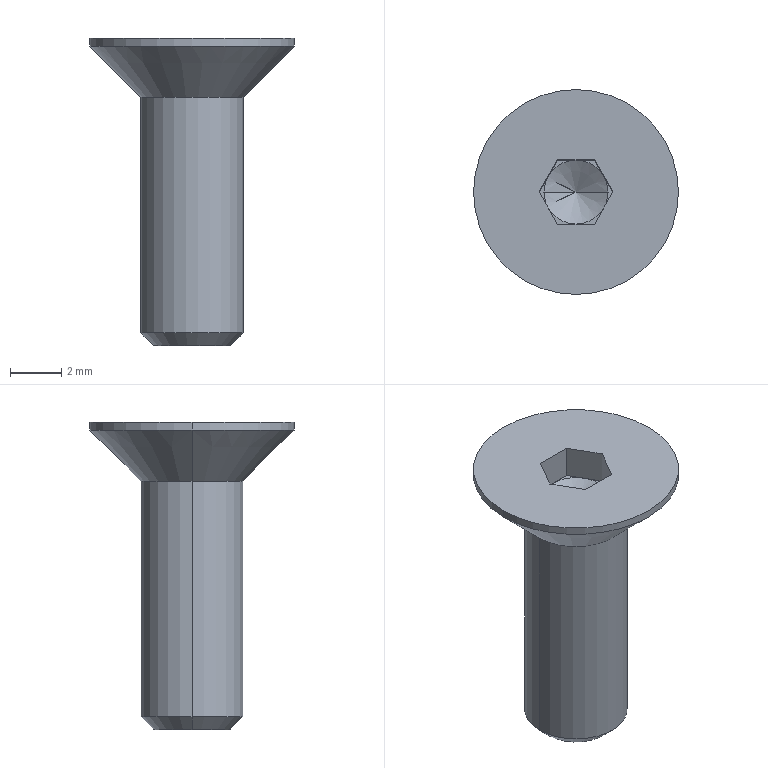Part | NX | features BREP 1 | 1 solid | 24 faces | box 8 x 8 x 12 mm | volume 185.959 mm3 | plane 14 | cone 6 | cylinder 4 | commonest cylinder face diameters 4 x2 8 x2
STEP:
#1=CARTESIAN_POINT('',(0.,0.,-2.022));
#2=VERTEX_POINT('',#1);
#3=CARTESIAN_POINT('',(-1.25,0.,-1.3));
#4=VERTEX_POINT('',#3);
#5=CARTESIAN_POINT('',(-1.25,0.,-1.3));
#6=DIRECTION('',(-0.866,0.,0.5));
#7=VECTOR('',#6,1000.);
#8=LINE('',#5,#7);
#9=EDGE_CURVE('',#2,#4,#8,.T.);
#10=ORIENTED_EDGE('',*,*,#9,.F.);
#11=CARTESIAN_POINT('',(1.25,0.,-1.3));
#12=VERTEX_POINT('',#11);
#13=CARTESIAN_POINT('',(1.25,0.,-1.3));
#14=DIRECTION('',(0.866,0.,0.5));
#15=VECTOR('',#14,1000.);
#16=LINE('',#13,#15);
#17=EDGE_CURVE('',#2,#12,#16,.T.);
#18=ORIENTED_EDGE('',*,*,#17,.T.);
#19=CARTESIAN_POINT('',(1.083,0.625,-1.3));
#20=VERTEX_POINT('',#19);
#21=CARTESIAN_POINT('',(0.,0.,-1.3));
#22=DIRECTION('',(0.,0.,-1.));
#23=DIRECTION('',(-1.,0.,0.));
#24=AXIS2_PLACEMENT_3D('',#21,#22,#23);
#25=CIRCLE('',#24,1.25);
#26=EDGE_CURVE('',#20,#12,#25,.T.);
#27=ORIENTED_EDGE('',*,*,#26,.F.);
#28=CARTESIAN_POINT('',(0.,1.25,-1.3));
#29=VERTEX_POINT('',#28);
#30=CARTESIAN_POINT('',(0.,0.,-1.3));
#31=DIRECTION('',(0.,0.,-1.));
#32=DIRECTION('',(-1.,0.,0.));
#33=AXIS2_PLACEMENT_3D('',#30,#31,#32);
#34=CIRCLE('',#33,1.25);
#35=EDGE_CURVE('',#29,#20,#34,.T.);
#36=ORIENTED_EDGE('',*,*,#35,.F.);
#37=CARTESIAN_POINT('',(-1.083,0.625,-1.3));
#38=VERTEX_POINT('',#37);
#39=CARTESIAN_POINT('',(0.,0.,-1.3));
#40=DIRECTION('',(0.,0.,-1.));
#41=DIRECTION('',(-1.,0.,0.));
#42=AXIS2_PLACEMENT_3D('',#39,#40,#41);
#43=CIRCLE('',#42,1.25);
#44=EDGE_CURVE('',#38,#29,#43,.T.);
#45=ORIENTED_EDGE('',*,*,#44,.F.);
#46=CARTESIAN_POINT('',(0.,0.,-1.3));
#47=DIRECTION('',(0.,0.,-1.));
#48=DIRECTION('',(-1.,0.,0.));
#49=AXIS2_PLACEMENT_3D('',#46,#47,#48);
#50=CIRCLE('',#49,1.25);
#51=EDGE_CURVE('',#4,#38,#50,.T.);
#52=ORIENTED_EDGE('',*,*,#51,.F.);
#53=EDGE_LOOP('',(#10,#18,#27,#36,#45,#52));
#54=FACE_BOUND('',#53,.T.);
#55=CARTESIAN_POINT('',(0.,0.,-1.3));
#56=DIRECTION('',(0.,0.,1.));
#57=DIRECTION('',(-1.,0.,0.));
#58=AXIS2_PLACEMENT_3D('',#55,#56,#57);
#59=CONICAL_SURFACE('',#58,1.25,1.047);
#60=ADVANCED_FACE('',(#54),#59,.F.);
#61=CARTESIAN_POINT('',(-1.5,0.,-12.));
#62=VERTEX_POINT('',#61);
#63=CARTESIAN_POINT('',(1.5,0.,-12.));
#64=VERTEX_POINT('',#63);
#65=CARTESIAN_POINT('',(0.,0.,-12.));
#66=DIRECTION('',(0.,0.,1.));
#67=DIRECTION('',(1.,0.,0.));
#68=AXIS2_PLACEMENT_3D('',#65,#66,#67);
#69=CIRCLE('',#68,1.5);
#70=EDGE_CURVE('',#62,#64,#69,.T.);
#71=ORIENTED_EDGE('',*,*,#70,.T.);
#72=CARTESIAN_POINT('',(2.,0.,-11.5));
#73=VERTEX_POINT('',#72);
#74=CARTESIAN_POINT('',(1.5,0.,-12.));
#75=DIRECTION('',(0.7071,0.,0.7071));
#76=VECTOR('',#75,1000.);
#77=LINE('',#74,#76);
#78=EDGE_CURVE('',#64,#73,#77,.T.);
#79=ORIENTED_EDGE('',*,*,#78,.T.);
#80=CARTESIAN_POINT('',(-2.,0.,-11.5));
#81=VERTEX_POINT('',#80);
#82=CARTESIAN_POINT('',(0.,0.,-11.5));
#83=DIRECTION('',(0.,0.,-1.));
#84=DIRECTION('',(1.,0.,0.));
#85=AXIS2_PLACEMENT_3D('',#82,#83,#84);
#86=CIRCLE('',#85,2.);
#87=EDGE_CURVE('',#73,#81,#86,.T.);
#88=ORIENTED_EDGE('',*,*,#87,.T.);
#89=CARTESIAN_POINT('',(-1.5,0.,-12.));
#90=DIRECTION('',(-0.7071,0.,0.7071));
#91=VECTOR('',#90,1000.);
#92=LINE('',#89,#91);
#93=EDGE_CURVE('',#62,#81,#92,.T.);
#94=ORIENTED_EDGE('',*,*,#93,.F.);
#95=EDGE_LOOP('',(#71,#79,#88,#94));
#96=FACE_BOUND('',#95,.T.);
#97=CARTESIAN_POINT('',(0.,0.,-12.));
#98=DIRECTION('',(0.,0.,1.));
#99=DIRECTION('',(-1.,0.,0.));
#100=AXIS2_PLACEMENT_3D('',#97,#98,#99);
#101=CONICAL_SURFACE('',#100,1.5,0.7854);
#102=ADVANCED_FACE('',(#96),#101,.T.);
#103=ORIENTED_EDGE('',*,*,#87,.F.);
#104=CARTESIAN_POINT('',(2.,0.,-2.3));
#105=VERTEX_POINT('',#104);
#106=CARTESIAN_POINT('',(2.,0.,-12.));
#107=DIRECTION('',(0.,0.,1.));
#108=VECTOR('',#107,1000.);
#109=LINE('',#106,#108);
#110=EDGE_CURVE('',#73,#105,#109,.T.);
#111=ORIENTED_EDGE('',*,*,#110,.T.);
#112=CARTESIAN_POINT('',(-2.,0.,-2.3));
#113=VERTEX_POINT('',#112);
#114=CARTESIAN_POINT('',(0.,0.,-2.3));
#115=DIRECTION('',(0.,0.,1.));
#116=DIRECTION('',(1.,0.,0.));
#117=AXIS2_PLACEMENT_3D('',#114,#115,#116);
#118=CIRCLE('',#117,2.);
#119=EDGE_CURVE('',#113,#105,#118,.T.);
#120=ORIENTED_EDGE('',*,*,#119,.F.);
#121=CARTESIAN_POINT('',(-2.,0.,-12.));
#122=DIRECTION('',(0.,0.,1.));
#123=VECTOR('',#122,1000.);
#124=LINE('',#121,#123);
#125=EDGE_CURVE('',#81,#113,#124,.T.);
#126=ORIENTED_EDGE('',*,*,#125,.F.);
#127=EDGE_LOOP('',(#103,#111,#120,#126));
#128=FACE_BOUND('',#127,.T.);
#129=CARTESIAN_POINT('',(0.,0.,-12.));
#130=DIRECTION('',(0.,0.,1.));
#131=DIRECTION('',(-1.,0.,0.));
#132=AXIS2_PLACEMENT_3D('',#129,#130,#131);
#133=CYLINDRICAL_SURFACE('',#132,2.);
#134=ADVANCED_FACE('',(#128),#133,.T.);
#135=ORIENTED_EDGE('',*,*,#119,.T.);
#136=CARTESIAN_POINT('',(4.,0.,-0.3));
#137=VERTEX_POINT('',#136);
#138=CARTESIAN_POINT('',(2.,0.,-2.3));
#139=DIRECTION('',(0.7071,0.,0.7071));
#140=VECTOR('',#139,1000.);
#141=LINE('',#138,#140);
#142=EDGE_CURVE('',#105,#137,#141,.T.);
#143=ORIENTED_EDGE('',*,*,#142,.T.);
#144=CARTESIAN_POINT('',(-4.,0.,-0.3));
#145=VERTEX_POINT('',#144);
#146=CARTESIAN_POINT('',(0.,0.,-0.3));
#147=DIRECTION('',(0.,0.,-1.));
#148=DIRECTION('',(1.,0.,0.));
#149=AXIS2_PLACEMENT_3D('',#146,#147,#148);
#150=CIRCLE('',#149,4.);
#151=EDGE_CURVE('',#137,#145,#150,.T.);
#152=ORIENTED_EDGE('',*,*,#151,.T.);
#153=CARTESIAN_POINT('',(-2.,0.,-2.3));
#154=DIRECTION('',(-0.7071,0.,0.7071));
#155=VECTOR('',#154,1000.);
#156=LINE('',#153,#155);
#157=EDGE_CURVE('',#113,#145,#156,.T.);
#158=ORIENTED_EDGE('',*,*,#157,.F.);
#159=EDGE_LOOP('',(#135,#143,#152,#158));
#160=FACE_BOUND('',#159,.T.);
#161=CARTESIAN_POINT('',(0.,0.,-2.3));
#162=DIRECTION('',(0.,0.,1.));
#163=DIRECTION('',(-1.,0.,0.));
#164=AXIS2_PLACEMENT_3D('',#161,#162,#163);
#165=CONICAL_SURFACE('',#164,2.,0.7854);
#166=ADVANCED_FACE('',(#160),#165,.T.);
#167=ORIENTED_EDGE('',*,*,#151,.F.);
#168=CARTESIAN_POINT('',(4.,0.,0.));
#169=VERTEX_POINT('',#168);
#170=CARTESIAN_POINT('',(4.,0.,-2.3));
#171=DIRECTION('',(0.,0.,1.));
#172=VECTOR('',#171,1000.);
#173=LINE('',#170,#172);
#174=EDGE_CURVE('',#137,#169,#173,.T.);
#175=ORIENTED_EDGE('',*,*,#174,.T.);
#176=CARTESIAN_POINT('',(-4.,0.,0.));
#177=VERTEX_POINT('',#176);
#178=CARTESIAN_POINT('',(0.,0.,0.));
#179=DIRECTION('',(0.,0.,1.));
#180=DIRECTION('',(1.,0.,0.));
#181=AXIS2_PLACEMENT_3D('',#178,#179,#180);
#182=CIRCLE('',#181,4.);
#183=EDGE_CURVE('',#177,#169,#182,.T.);
#184=ORIENTED_EDGE('',*,*,#183,.F.);
#185=CARTESIAN_POINT('',(-4.,0.,-2.3));
#186=DIRECTION('',(0.,0.,1.));
#187=VECTOR('',#186,1000.);
#188=LINE('',#185,#187);
#189=EDGE_CURVE('',#145,#177,#188,.T.);
#190=ORIENTED_EDGE('',*,*,#189,.F.);
#191=EDGE_LOOP('',(#167,#175,#184,#190));
#192=FACE_BOUND('',#191,.T.);
#193=CARTESIAN_POINT('',(0.,0.,-2.3));
#194=DIRECTION('',(0.,0.,1.));
#195=DIRECTION('',(-1.,0.,0.));
#196=AXIS2_PLACEMENT_3D('',#193,#194,#195);
#197=CYLINDRICAL_SURFACE('',#196,4.);
#198=ADVANCED_FACE('',(#192),#197,.T.);
#199=ORIENTED_EDGE('',*,*,#44,.T.);
#200=CARTESIAN_POINT('',(-0.7217,1.25,-1.3));
#201=VERTEX_POINT('',#200);
#202=CARTESIAN_POINT('',(-0.7217,1.25,-1.3));
#203=DIRECTION('',(1.,0.,0.));
#204=VECTOR('',#203,1000.);
#205=LINE('',#202,#204);
#206=EDGE_CURVE('',#201,#29,#205,.T.);
#207=ORIENTED_EDGE('',*,*,#206,.F.);
#208=CARTESIAN_POINT('',(-1.443,0.,-1.3));
#209=DIRECTION('',(0.5,0.866,0.));
#210=VECTOR('',#209,1000.);
#211=LINE('',#208,#210);
#212=EDGE_CURVE('',#38,#201,#211,.T.);
#213=ORIENTED_EDGE('',*,*,#212,.F.);
#214=EDGE_LOOP('',(#199,#207,#213));
#215=FACE_BOUND('',#214,.T.);
#216=CARTESIAN_POINT('',(0.,0.,-1.3));
#217=DIRECTION('',(0.,0.,1.));
#218=DIRECTION('',(1.,0.,0.));
#219=AXIS2_PLACEMENT_3D('',#216,#217,#218);
#220=PLANE('',#219);
#221=ADVANCED_FACE('',(#215),#220,.T.);
#222=ORIENTED_EDGE('',*,*,#35,.T.);
#223=CARTESIAN_POINT('',(0.7217,1.25,-1.3));
#224=VERTEX_POINT('',#223);
#225=CARTESIAN_POINT('',(0.7217,1.25,-1.3));
#226=DIRECTION('',(0.5,-0.866,0.));
#227=VECTOR('',#226,1000.);
#228=LINE('',#225,#227);
#229=EDGE_CURVE('',#224,#20,#228,.T.);
#230=ORIENTED_EDGE('',*,*,#229,.F.);
#231=CARTESIAN_POINT('',(-0.7217,1.25,-1.3));
#232=DIRECTION('',(1.,0.,0.));
#233=VECTOR('',#232,1000.);
#234=LINE('',#231,#233);
#235=EDGE_CURVE('',#29,#224,#234,.T.);
#236=ORIENTED_EDGE('',*,*,#235,.F.);
#237=EDGE_LOOP('',(#222,#230,#236));
#238=FACE_BOUND('',#237,.T.);
#239=CARTESIAN_POINT('',(0.,0.,-1.3));
#240=DIRECTION('',(0.,0.,1.));
#241=DIRECTION('',(1.,0.,0.));
#242=AXIS2_PLACEMENT_3D('',#239,#240,#241);
#243=PLANE('',#242);
#244=ADVANCED_FACE('',(#238),#243,.T.);
#245=ORIENTED_EDGE('',*,*,#26,.T.);
#246=CARTESIAN_POINT('',(1.083,-0.625,-1.3));
#247=VERTEX_POINT('',#246);
#248=CARTESIAN_POINT('',(0.,0.,-1.3));
#249=DIRECTION('',(0.,0.,-1.));
#250=DIRECTION('',(-1.,0.,0.));
#251=AXIS2_PLACEMENT_3D('',#248,#249,#250);
#252=CIRCLE('',#251,1.25);
#253=EDGE_CURVE('',#12,#247,#252,.T.);
#254=ORIENTED_EDGE('',*,*,#253,.T.);
#255=CARTESIAN_POINT('',(1.443,0.,-1.3));
#256=VERTEX_POINT('',#255);
#257=CARTESIAN_POINT('',(1.443,0.,-1.3));
#258=DIRECTION('',(-0.5,-0.866,0.));
#259=VECTOR('',#258,1000.);
#260=LINE('',#257,#259);
#261=EDGE_CURVE('',#256,#247,#260,.T.);
#262=ORIENTED_EDGE('',*,*,#261,.F.);
#263=CARTESIAN_POINT('',(0.7217,1.25,-1.3));
#264=DIRECTION('',(0.5,-0.866,0.));
#265=VECTOR('',#264,1000.);
#266=LINE('',#263,#265);
#267=EDGE_CURVE('',#20,#256,#266,.T.);
#268=ORIENTED_EDGE('',*,*,#267,.F.);
#269=EDGE_LOOP('',(#245,#254,#262,#268));
#270=FACE_BOUND('',#269,.T.);
#271=CARTESIAN_POINT('',(0.,0.,-1.3));
#272=DIRECTION('',(0.,0.,1.));
#273=DIRECTION('',(1.,0.,0.));
#274=AXIS2_PLACEMENT_3D('',#271,#272,#273);
#275=PLANE('',#274);
#276=ADVANCED_FACE('',(#270),#275,.T.);
#277=CARTESIAN_POINT('',(0.,-1.25,-1.3));
#278=VERTEX_POINT('',#277);
#279=CARTESIAN_POINT('',(0.,0.,-1.3));
#280=DIRECTION('',(0.,0.,-1.));
#281=DIRECTION('',(-1.,0.,0.));
#282=AXIS2_PLACEMENT_3D('',#279,#280,#281);
#283=CIRCLE('',#282,1.25);
#284=EDGE_CURVE('',#247,#278,#283,.T.);
#285=ORIENTED_EDGE('',*,*,#284,.T.);
#286=CARTESIAN_POINT('',(0.7217,-1.25,-1.3));
#287=VERTEX_POINT('',#286);
#288=CARTESIAN_POINT('',(0.7217,-1.25,-1.3));
#289=DIRECTION('',(-1.,0.,0.));
#290=VECTOR('',#289,1000.);
#291=LINE('',#288,#290);
#292=EDGE_CURVE('',#287,#278,#291,.T.);
#293=ORIENTED_EDGE('',*,*,#292,.F.);
#294=CARTESIAN_POINT('',(1.443,0.,-1.3));
#295=DIRECTION('',(-0.5,-0.866,0.));
#296=VECTOR('',#295,1000.);
#297=LINE('',#294,#296);
#298=EDGE_CURVE('',#247,#287,#297,.T.);
#299=ORIENTED_EDGE('',*,*,#298,.F.);
#300=EDGE_LOOP('',(#285,#293,#299));
#301=FACE_BOUND('',#300,.T.);
#302=CARTESIAN_POINT('',(0.,0.,-1.3));
#303=DIRECTION('',(0.,0.,1.));
#304=DIRECTION('',(1.,0.,0.));
#305=AXIS2_PLACEMENT_3D('',#302,#303,#304);
#306=PLANE('',#305);
#307=ADVANCED_FACE('',(#301),#306,.T.);
#308=CARTESIAN_POINT('',(-1.083,-0.625,-1.3));
#309=VERTEX_POINT('',#308);
#310=CARTESIAN_POINT('',(0.,0.,-1.3));
#311=DIRECTION('',(0.,0.,-1.));
#312=DIRECTION('',(-1.,0.,0.));
#313=AXIS2_PLACEMENT_3D('',#310,#311,#312);
#314=CIRCLE('',#313,1.25);
#315=EDGE_CURVE('',#278,#309,#314,.T.);
#316=ORIENTED_EDGE('',*,*,#315,.T.);
#317=CARTESIAN_POINT('',(-0.7217,-1.25,-1.3));
#318=VERTEX_POINT('',#317);
#319=CARTESIAN_POINT('',(-0.7217,-1.25,-1.3));
#320=DIRECTION('',(-0.5,0.866,0.));
#321=VECTOR('',#320,1000.);
#322=LINE('',#319,#321);
#323=EDGE_CURVE('',#318,#309,#322,.T.);
#324=ORIENTED_EDGE('',*,*,#323,.F.);
#325=CARTESIAN_POINT('',(0.7217,-1.25,-1.3));
#326=DIRECTION('',(-1.,0.,0.));
#327=VECTOR('',#326,1000.);
#328=LINE('',#325,#327);
#329=EDGE_CURVE('',#278,#318,#328,.T.);
#330=ORIENTED_EDGE('',*,*,#329,.F.);
#331=EDGE_LOOP('',(#316,#324,#330));
#332=FACE_BOUND('',#331,.T.);
#333=CARTESIAN_POINT('',(0.,0.,-1.3));
#334=DIRECTION('',(0.,0.,1.));
#335=DIRECTION('',(1.,0.,0.));
#336=AXIS2_PLACEMENT_3D('',#333,#334,#335);
#337=PLANE('',#336);
#338=ADVANCED_FACE('',(#332),#337,.T.);
#339=ORIENTED_EDGE('',*,*,#174,.F.);
#340=CARTESIAN_POINT('',(0.,0.,-0.3));
#341=DIRECTION('',(0.,0.,-1.));
#342=DIRECTION('',(1.,0.,0.));
#343=AXIS2_PLACEMENT_3D('',#340,#341,#342);
#344=CIRCLE('',#343,4.);
#345=EDGE_CURVE('',#145,#137,#344,.T.);
#346=ORIENTED_EDGE('',*,*,#345,.F.);
#347=ORIENTED_EDGE('',*,*,#189,.T.);
#348=CARTESIAN_POINT('',(0.,0.,0.));
#349=DIRECTION('',(0.,0.,1.));
#350=DIRECTION('',(1.,0.,0.));
#351=AXIS2_PLACEMENT_3D('',#348,#349,#350);
#352=CIRCLE('',#351,4.);
#353=EDGE_CURVE('',#169,#177,#352,.T.);
#354=ORIENTED_EDGE('',*,*,#353,.F.);
#355=EDGE_LOOP('',(#339,#346,#347,#354));
#356=FACE_BOUND('',#355,.T.);
#357=CARTESIAN_POINT('',(0.,0.,-2.3));
#358=DIRECTION('',(0.,0.,1.));
#359=DIRECTION('',(-1.,0.,0.));
#360=AXIS2_PLACEMENT_3D('',#357,#358,#359);
#361=CYLINDRICAL_SURFACE('',#360,4.);
#362=ADVANCED_FACE('',(#356),#361,.T.);
#363=ORIENTED_EDGE('',*,*,#183,.T.);
#364=ORIENTED_EDGE('',*,*,#353,.T.);
#365=EDGE_LOOP('',(#363,#364));
#366=FACE_BOUND('',#365,.T.);
#367=CARTESIAN_POINT('',(-0.7217,1.25,0.));
#368=VERTEX_POINT('',#367);
#369=CARTESIAN_POINT('',(0.7217,1.25,0.));
#370=VERTEX_POINT('',#369);
#371=CARTESIAN_POINT('',(-0.7217,1.25,0.));
#372=DIRECTION('',(1.,0.,0.));
#373=VECTOR('',#372,1000.);
#374=LINE('',#371,#373);
#375=EDGE_CURVE('',#368,#370,#374,.T.);
#376=ORIENTED_EDGE('',*,*,#375,.T.);
#377=CARTESIAN_POINT('',(1.443,0.,0.));
#378=VERTEX_POINT('',#377);
#379=CARTESIAN_POINT('',(0.7217,1.25,0.));
#380=DIRECTION('',(0.5,-0.866,0.));
#381=VECTOR('',#380,1000.);
#382=LINE('',#379,#381);
#383=EDGE_CURVE('',#370,#378,#382,.T.);
#384=ORIENTED_EDGE('',*,*,#383,.T.);
#385=CARTESIAN_POINT('',(0.7217,-1.25,0.));
#386=VERTEX_POINT('',#385);
#387=CARTESIAN_POINT('',(1.443,0.,0.));
#388=DIRECTION('',(-0.5,-0.866,0.));
#389=VECTOR('',#388,1000.);
#390=LINE('',#387,#389);
#391=EDGE_CURVE('',#378,#386,#390,.T.);
#392=ORIENTED_EDGE('',*,*,#391,.T.);
#393=CARTESIAN_POINT('',(-0.7217,-1.25,0.));
#394=VERTEX_POINT('',#393);
#395=CARTESIAN_POINT('',(0.7217,-1.25,0.));
#396=DIRECTION('',(-1.,0.,0.));
#397=VECTOR('',#396,1000.);
#398=LINE('',#395,#397);
#399=EDGE_CURVE('',#386,#394,#398,.T.);
#400=ORIENTED_EDGE('',*,*,#399,.T.);
#401=CARTESIAN_POINT('',(-1.443,0.,0.));
#402=VERTEX_POINT('',#401);
#403=CARTESIAN_POINT('',(-0.7217,-1.25,0.));
#404=DIRECTION('',(-0.5,0.866,0.));
#405=VECTOR('',#404,1000.);
#406=LINE('',#403,#405);
#407=EDGE_CURVE('',#394,#402,#406,.T.);
#408=ORIENTED_EDGE('',*,*,#407,.T.);
#409=CARTESIAN_POINT('',(-1.443,0.,0.));
#410=DIRECTION('',(0.5,0.866,0.));
#411=VECTOR('',#410,1000.);
#412=LINE('',#409,#411);
#413=EDGE_CURVE('',#402,#368,#412,.T.);
#414=ORIENTED_EDGE('',*,*,#413,.T.);
#415=EDGE_LOOP('',(#376,#384,#392,#400,#408,#414));
#416=FACE_BOUND('',#415,.T.);
#417=CARTESIAN_POINT('',(0.,0.,0.));
#418=DIRECTION('',(0.,0.,-1.));
#419=DIRECTION('',(0.,-1.,0.));
#420=AXIS2_PLACEMENT_3D('',#417,#418,#419);
#421=PLANE('',#420);
#422=ADVANCED_FACE('',(#366,#416),#421,.F.);
#423=ORIENTED_EDGE('',*,*,#142,.F.);
#424=CARTESIAN_POINT('',(0.,0.,-2.3));
#425=DIRECTION('',(0.,0.,1.));
#426=DIRECTION('',(1.,0.,0.));
#427=AXIS2_PLACEMENT_3D('',#424,#425,#426);
#428=CIRCLE('',#427,2.);
#429=EDGE_CURVE('',#105,#113,#428,.T.);
#430=ORIENTED_EDGE('',*,*,#429,.T.);
#431=ORIENTED_EDGE('',*,*,#157,.T.);
#432=ORIENTED_EDGE('',*,*,#345,.T.);
#433=EDGE_LOOP('',(#423,#430,#431,#432));
#434=FACE_BOUND('',#433,.T.);
#435=CARTESIAN_POINT('',(0.,0.,-2.3));
#436=DIRECTION('',(0.,0.,1.));
#437=DIRECTION('',(-1.,0.,0.));
#438=AXIS2_PLACEMENT_3D('',#435,#436,#437);
#439=CONICAL_SURFACE('',#438,2.,0.7854);
#440=ADVANCED_FACE('',(#434),#439,.T.);
#441=ORIENTED_EDGE('',*,*,#110,.F.);
#442=CARTESIAN_POINT('',(0.,0.,-11.5));
#443=DIRECTION('',(0.,0.,-1.));
#444=DIRECTION('',(1.,0.,0.));
#445=AXIS2_PLACEMENT_3D('',#442,#443,#444);
#446=CIRCLE('',#445,2.);
#447=EDGE_CURVE('',#81,#73,#446,.T.);
#448=ORIENTED_EDGE('',*,*,#447,.F.);
#449=ORIENTED_EDGE('',*,*,#125,.T.);
#450=ORIENTED_EDGE('',*,*,#429,.F.);
#451=EDGE_LOOP('',(#441,#448,#449,#450));
#452=FACE_BOUND('',#451,.T.);
#453=CARTESIAN_POINT('',(0.,0.,-12.));
#454=DIRECTION('',(0.,0.,1.));
#455=DIRECTION('',(-1.,0.,0.));
#456=AXIS2_PLACEMENT_3D('',#453,#454,#455);
#457=CYLINDRICAL_SURFACE('',#456,2.);
#458=ADVANCED_FACE('',(#452),#457,.T.);
#459=ORIENTED_EDGE('',*,*,#70,.F.);
#460=CARTESIAN_POINT('',(0.,0.,-12.));
#461=DIRECTION('',(0.,0.,1.));
#462=DIRECTION('',(1.,0.,0.));
#463=AXIS2_PLACEMENT_3D('',#460,#461,#462);
#464=CIRCLE('',#463,1.5);
#465=EDGE_CURVE('',#64,#62,#464,.T.);
#466=ORIENTED_EDGE('',*,*,#465,.F.);
#467=EDGE_LOOP('',(#459,#466));
#468=FACE_BOUND('',#467,.T.);
#469=CARTESIAN_POINT('',(0.,0.,-12.));
#470=DIRECTION('',(0.,0.,-1.));
#471=DIRECTION('',(0.,-1.,0.));
#472=AXIS2_PLACEMENT_3D('',#469,#470,#471);
#473=PLANE('',#472);
#474=ADVANCED_FACE('',(#468),#473,.T.);
#475=ORIENTED_EDGE('',*,*,#78,.F.);
#476=ORIENTED_EDGE('',*,*,#465,.T.);
#477=ORIENTED_EDGE('',*,*,#93,.T.);
#478=ORIENTED_EDGE('',*,*,#447,.T.);
#479=EDGE_LOOP('',(#475,#476,#477,#478));
#480=FACE_BOUND('',#479,.T.);
#481=CARTESIAN_POINT('',(0.,0.,-12.));
#482=DIRECTION('',(0.,0.,1.));
#483=DIRECTION('',(-1.,0.,0.));
#484=AXIS2_PLACEMENT_3D('',#481,#482,#483);
#485=CONICAL_SURFACE('',#484,1.5,0.7854);
#486=ADVANCED_FACE('',(#480),#485,.T.);
#487=ORIENTED_EDGE('',*,*,#413,.F.);
#488=CARTESIAN_POINT('',(-1.443,0.,-1.3));
#489=VERTEX_POINT('',#488);
#490=CARTESIAN_POINT('',(-1.443,0.,-1.3));
#491=DIRECTION('',(0.,0.,1.));
#492=VECTOR('',#491,1000.);
#493=LINE('',#490,#492);
#494=EDGE_CURVE('',#489,#402,#493,.T.);
#495=ORIENTED_EDGE('',*,*,#494,.F.);
#496=CARTESIAN_POINT('',(-1.443,0.,-1.3));
#497=DIRECTION('',(0.5,0.866,0.));
#498=VECTOR('',#497,1000.);
#499=LINE('',#496,#498);
#500=EDGE_CURVE('',#489,#38,#499,.T.);
#501=ORIENTED_EDGE('',*,*,#500,.T.);
#502=ORIENTED_EDGE('',*,*,#212,.T.);
#503=CARTESIAN_POINT('',(-0.7217,1.25,-1.3));
#504=DIRECTION('',(0.,0.,1.));
#505=VECTOR('',#504,1000.);
#506=LINE('',#503,#505);
#507=EDGE_CURVE('',#201,#368,#506,.T.);
#508=ORIENTED_EDGE('',*,*,#507,.T.);
#509=EDGE_LOOP('',(#487,#495,#501,#502,#508));
#510=FACE_BOUND('',#509,.T.);
#511=CARTESIAN_POINT('',(-1.443,0.,-1.3));
#512=DIRECTION('',(-0.866,0.5,0.));
#513=DIRECTION('',(0.,0.,1.));
#514=AXIS2_PLACEMENT_3D('',#511,#512,#513);
#515=PLANE('',#514);
#516=ADVANCED_FACE('',(#510),#515,.F.);
#517=ORIENTED_EDGE('',*,*,#407,.F.);
#518=CARTESIAN_POINT('',(-0.7217,-1.25,-1.3));
#519=DIRECTION('',(0.,0.,1.));
#520=VECTOR('',#519,1000.);
#521=LINE('',#518,#520);
#522=EDGE_CURVE('',#318,#394,#521,.T.);
#523=ORIENTED_EDGE('',*,*,#522,.F.);
#524=ORIENTED_EDGE('',*,*,#323,.T.);
#525=CARTESIAN_POINT('',(-0.7217,-1.25,-1.3));
#526=DIRECTION('',(-0.5,0.866,0.));
#527=VECTOR('',#526,1000.);
#528=LINE('',#525,#527);
#529=EDGE_CURVE('',#309,#489,#528,.T.);
#530=ORIENTED_EDGE('',*,*,#529,.T.);
#531=ORIENTED_EDGE('',*,*,#494,.T.);
#532=EDGE_LOOP('',(#517,#523,#524,#530,#531));
#533=FACE_BOUND('',#532,.T.);
#534=CARTESIAN_POINT('',(-0.7217,-1.25,-1.3));
#535=DIRECTION('',(-0.866,-0.5,0.));
#536=DIRECTION('',(-0.5,0.866,0.));
#537=AXIS2_PLACEMENT_3D('',#534,#535,#536);
#538=PLANE('',#537);
#539=ADVANCED_FACE('',(#533),#538,.F.);
#540=ORIENTED_EDGE('',*,*,#399,.F.);
#541=CARTESIAN_POINT('',(0.7217,-1.25,-1.3));
#542=DIRECTION('',(0.,0.,1.));
#543=VECTOR('',#542,1000.);
#544=LINE('',#541,#543);
#545=EDGE_CURVE('',#287,#386,#544,.T.);
#546=ORIENTED_EDGE('',*,*,#545,.F.);
#547=ORIENTED_EDGE('',*,*,#292,.T.);
#548=ORIENTED_EDGE('',*,*,#329,.T.);
#549=ORIENTED_EDGE('',*,*,#522,.T.);
#550=EDGE_LOOP('',(#540,#546,#547,#548,#549));
#551=FACE_BOUND('',#550,.T.);
#552=CARTESIAN_POINT('',(0.7217,-1.25,-1.3));
#553=DIRECTION('',(0.,-1.,0.));
#554=DIRECTION('',(0.,0.,-1.));
#555=AXIS2_PLACEMENT_3D('',#552,#553,#554);
#556=PLANE('',#555);
#557=ADVANCED_FACE('',(#551),#556,.F.);
#558=ORIENTED_EDGE('',*,*,#391,.F.);
#559=CARTESIAN_POINT('',(1.443,0.,-1.3));
#560=DIRECTION('',(0.,0.,1.));
#561=VECTOR('',#560,1000.);
#562=LINE('',#559,#561);
#563=EDGE_CURVE('',#256,#378,#562,.T.);
#564=ORIENTED_EDGE('',*,*,#563,.F.);
#565=ORIENTED_EDGE('',*,*,#261,.T.);
#566=ORIENTED_EDGE('',*,*,#298,.T.);
#567=ORIENTED_EDGE('',*,*,#545,.T.);
#568=EDGE_LOOP('',(#558,#564,#565,#566,#567));
#569=FACE_BOUND('',#568,.T.);
#570=CARTESIAN_POINT('',(1.443,0.,-1.3));
#571=DIRECTION('',(0.866,-0.5,0.));
#572=DIRECTION('',(0.,0.,-1.));
#573=AXIS2_PLACEMENT_3D('',#570,#571,#572);
#574=PLANE('',#573);
#575=ADVANCED_FACE('',(#569),#574,.F.);
#576=ORIENTED_EDGE('',*,*,#383,.F.);
#577=CARTESIAN_POINT('',(0.7217,1.25,-1.3));
#578=DIRECTION('',(0.,0.,1.));
#579=VECTOR('',#578,1000.);
#580=LINE('',#577,#579);
#581=EDGE_CURVE('',#224,#370,#580,.T.);
#582=ORIENTED_EDGE('',*,*,#581,.F.);
#583=ORIENTED_EDGE('',*,*,#229,.T.);
#584=ORIENTED_EDGE('',*,*,#267,.T.);
#585=ORIENTED_EDGE('',*,*,#563,.T.);
#586=EDGE_LOOP('',(#576,#582,#583,#584,#585));
#587=FACE_BOUND('',#586,.T.);
#588=CARTESIAN_POINT('',(0.7217,1.25,-1.3));
#589=DIRECTION('',(0.866,0.5,0.));
#590=DIRECTION('',(0.,0.,-1.));
#591=AXIS2_PLACEMENT_3D('',#588,#589,#590);
#592=PLANE('',#591);
#593=ADVANCED_FACE('',(#587),#592,.F.);
#594=ORIENTED_EDGE('',*,*,#375,.F.);
#595=ORIENTED_EDGE('',*,*,#507,.F.);
#596=ORIENTED_EDGE('',*,*,#206,.T.);
#597=ORIENTED_EDGE('',*,*,#235,.T.);
#598=ORIENTED_EDGE('',*,*,#581,.T.);
#599=EDGE_LOOP('',(#594,#595,#596,#597,#598));
#600=FACE_BOUND('',#599,.T.);
#601=CARTESIAN_POINT('',(-0.7217,1.25,-1.3));
#602=DIRECTION('',(0.,1.,0.));
#603=DIRECTION('',(1.,0.,0.));
#604=AXIS2_PLACEMENT_3D('',#601,#602,#603);
#605=PLANE('',#604);
#606=ADVANCED_FACE('',(#600),#605,.F.);
#607=CARTESIAN_POINT('',(0.,0.,-1.3));
#608=DIRECTION('',(0.,0.,-1.));
#609=DIRECTION('',(-1.,0.,0.));
#610=AXIS2_PLACEMENT_3D('',#607,#608,#609);
#611=CIRCLE('',#610,1.25);
#612=EDGE_CURVE('',#309,#4,#611,.T.);
#613=ORIENTED_EDGE('',*,*,#612,.T.);
#614=ORIENTED_EDGE('',*,*,#51,.T.);
#615=ORIENTED_EDGE('',*,*,#500,.F.);
#616=ORIENTED_EDGE('',*,*,#529,.F.);
#617=EDGE_LOOP('',(#613,#614,#615,#616));
#618=FACE_BOUND('',#617,.T.);
#619=CARTESIAN_POINT('',(0.,0.,-1.3));
#620=DIRECTION('',(0.,0.,1.));
#621=DIRECTION('',(1.,0.,0.));
#622=AXIS2_PLACEMENT_3D('',#619,#620,#621);
#623=PLANE('',#622);
#624=ADVANCED_FACE('',(#618),#623,.T.);
#625=ORIENTED_EDGE('',*,*,#17,.F.);
#626=ORIENTED_EDGE('',*,*,#9,.T.);
#627=ORIENTED_EDGE('',*,*,#612,.F.);
#628=ORIENTED_EDGE('',*,*,#315,.F.);
#629=ORIENTED_EDGE('',*,*,#284,.F.);
#630=ORIENTED_EDGE('',*,*,#253,.F.);
#631=EDGE_LOOP('',(#625,#626,#627,#628,#629,#630));
#632=FACE_BOUND('',#631,.T.);
#633=CARTESIAN_POINT('',(0.,0.,-1.3));
#634=DIRECTION('',(0.,0.,1.));
#635=DIRECTION('',(-1.,0.,0.));
#636=AXIS2_PLACEMENT_3D('',#633,#634,#635);
#637=CONICAL_SURFACE('',#636,1.25,1.047);
#638=ADVANCED_FACE('',(#632),#637,.F.);
#639=CLOSED_SHELL('',(#60,#102,#134,#166,#198,#221,#244,#276,#307,#338,#362,#422,#440,#458,#474,#486,#516,#539,#557,#575,#593,#606,#624,#638));
#640=MANIFOLD_SOLID_BREP('',#639);
#641=(LENGTH_UNIT()NAMED_UNIT(*)SI_UNIT(.MILLI.,.METRE.));
#642=UNCERTAINTY_MEASURE_WITH_UNIT(LENGTH_MEASURE(0.00001),#641,'','');
#643=(NAMED_UNIT(*)PLANE_ANGLE_UNIT()SI_UNIT($,.RADIAN.));
#644=(NAMED_UNIT(*)SI_UNIT($,.STERADIAN.)SOLID_ANGLE_UNIT());
#645=(GEOMETRIC_REPRESENTATION_CONTEXT(3)GLOBAL_UNCERTAINTY_ASSIGNED_CONTEXT((#642))GLOBAL_UNIT_ASSIGNED_CONTEXT((#641,#643,#644))REPRESENTATION_CONTEXT('',''));
#646=ADVANCED_BREP_SHAPE_REPRESENTATION('',(#640),#645);